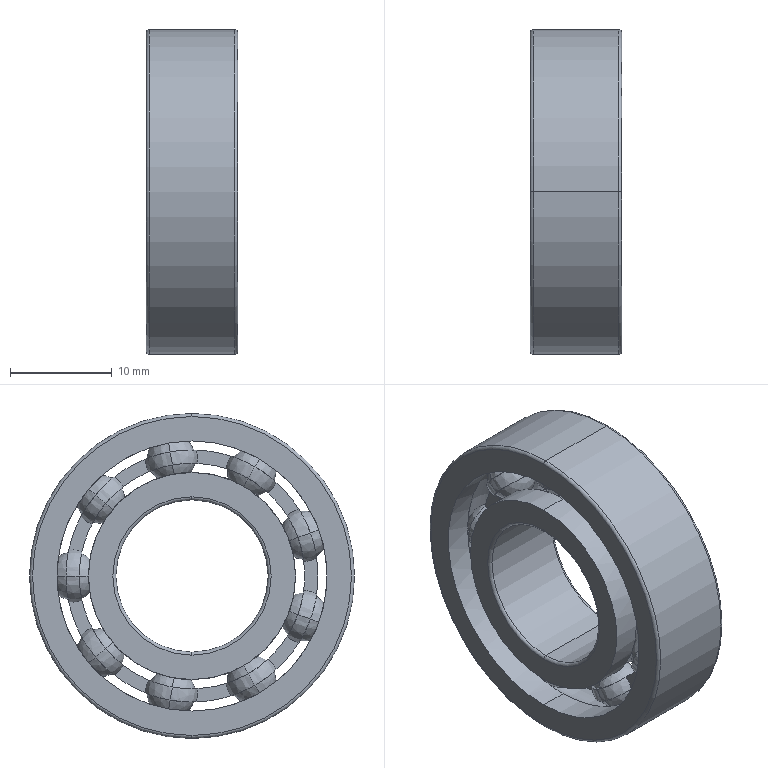Part | STEP file | Bearing 6002Z | 1 solid | 148 faces | box 9 x 32 x 32 mm | volume 3871 mm3 | sphere 72 | torus 38 | plane 22 | cylinder 16 | commonest cylinder face diameters 20.4 x4 26.6 x4 15 x2 22.19 x2 24.81 x2 32 x2